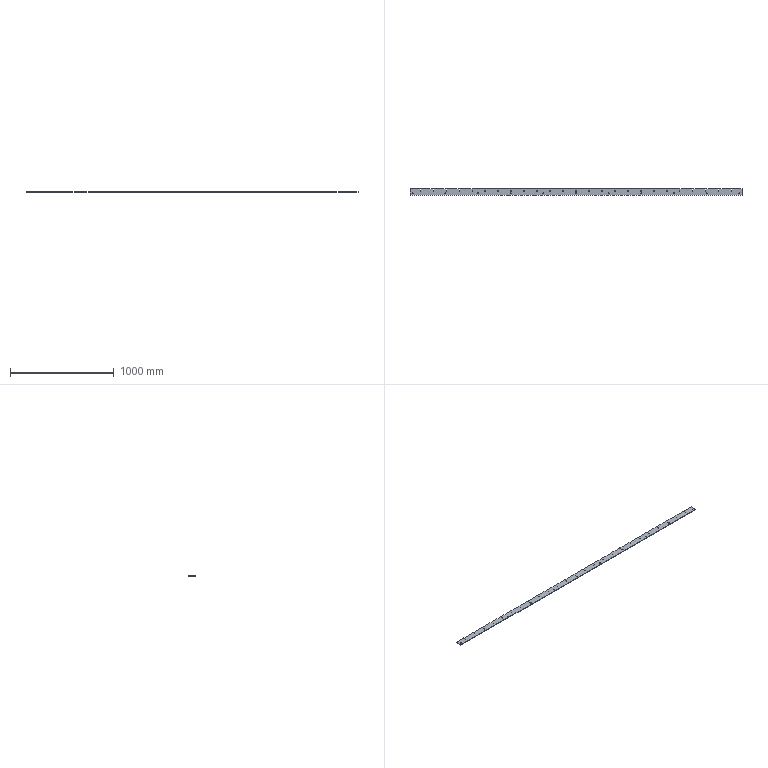Part | SolidWorks | features FlatPattern 1, HoleWzd 1, ICE 1, SMBaseFlange 1, SheetMetal 1 | 1 solid | 128 faces | box 3200 x 60 x 4.5 mm | volume 848029 mm3 | plane 106 | cylinder 22 | commonest cylinder face diameters 8.5 x22